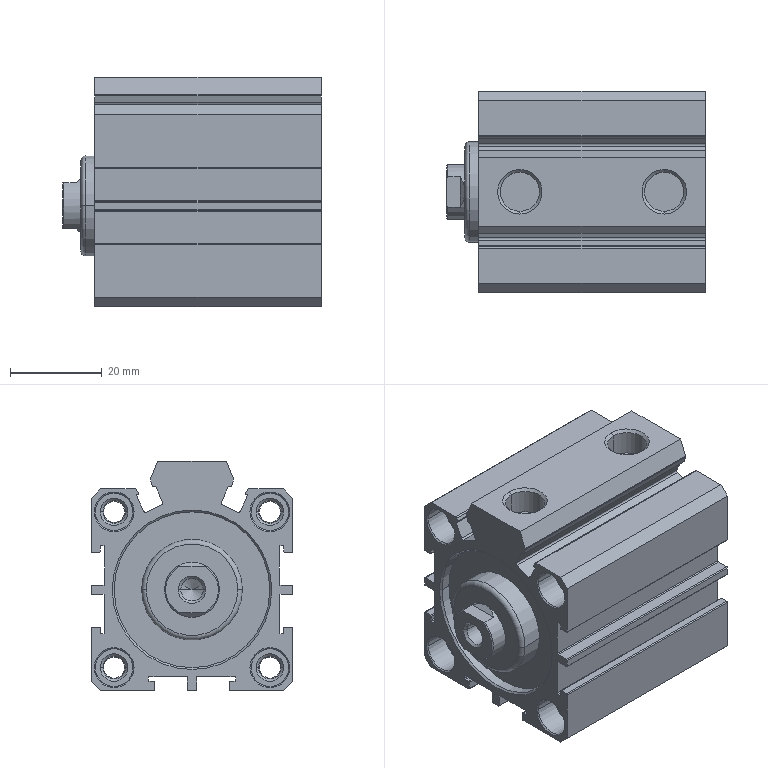Part | STEP file | slim cylinder SDA32x15S | 2 solids | 274 faces | box 56.5 x 44 x 50 mm | volume 73999 mm3 | cylinder 116 | plane 94 | cone 62 | torus 2 | commonest cylinder face diameters 0.4 x46 4.917 x18 8.2 x16 0.8 x10 4.6 x8 8.566 x4